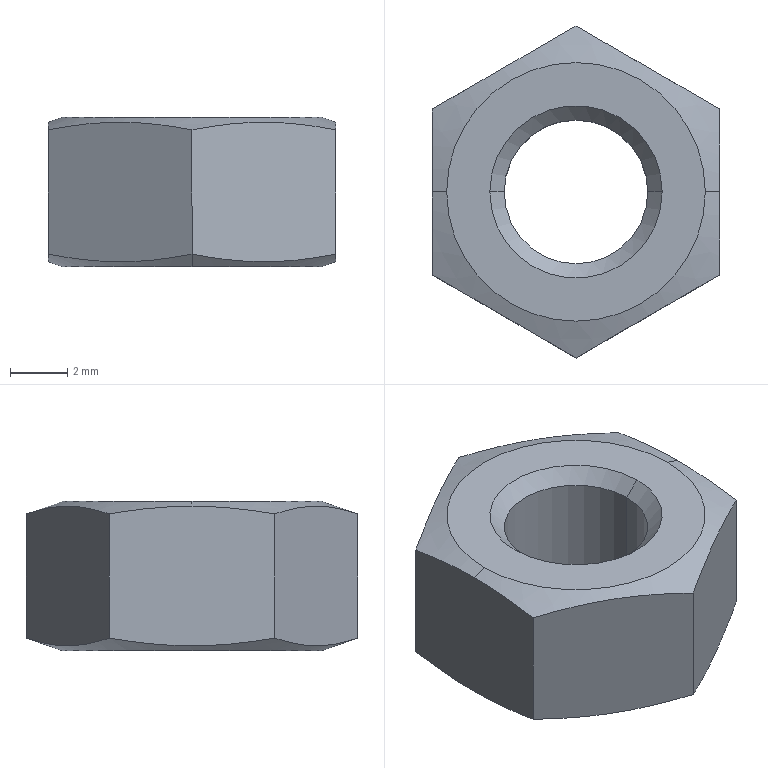Part | STEP file | 921271102 | 1 solid | 18 faces | box 10 x 11.547 x 5.2 mm | volume 337.323 mm3 | cone 8 | plane 8 | cylinder 2 | commonest cylinder face diameters 5 x2
STEP:
#1=CARTESIAN_POINT('',(2.5,0.,4.7));
#2=VERTEX_POINT('',#1);
#3=CARTESIAN_POINT('',(-2.5,0.,4.7));
#4=VERTEX_POINT('',#3);
#5=CARTESIAN_POINT('',(0.,0.,4.7));
#6=DIRECTION('',(0.,0.,-1.));
#7=DIRECTION('',(-1.,0.,0.));
#8=AXIS2_PLACEMENT_3D('',#5,#6,#7);
#9=CIRCLE('',#8,2.5);
#10=EDGE_CURVE('',#2,#4,#9,.T.);
#11=ORIENTED_EDGE('',*,*,#10,.F.);
#12=CARTESIAN_POINT('',(2.5,0.,0.5));
#13=VERTEX_POINT('',#12);
#14=CARTESIAN_POINT('',(2.5,0.,5.2));
#15=DIRECTION('',(0.,0.,-1.));
#16=VECTOR('',#15,1000.);
#17=LINE('',#14,#16);
#18=EDGE_CURVE('',#2,#13,#17,.T.);
#19=ORIENTED_EDGE('',*,*,#18,.T.);
#20=CARTESIAN_POINT('',(-2.5,0.,0.5));
#21=VERTEX_POINT('',#20);
#22=CARTESIAN_POINT('',(0.,0.,0.5));
#23=DIRECTION('',(0.,0.,1.));
#24=DIRECTION('',(-1.,0.,0.));
#25=AXIS2_PLACEMENT_3D('',#22,#23,#24);
#26=CIRCLE('',#25,2.5);
#27=EDGE_CURVE('',#21,#13,#26,.T.);
#28=ORIENTED_EDGE('',*,*,#27,.F.);
#29=CARTESIAN_POINT('',(-2.5,0.,5.2));
#30=DIRECTION('',(0.,0.,-1.));
#31=VECTOR('',#30,1000.);
#32=LINE('',#29,#31);
#33=EDGE_CURVE('',#4,#21,#32,.T.);
#34=ORIENTED_EDGE('',*,*,#33,.F.);
#35=EDGE_LOOP('',(#11,#19,#28,#34));
#36=FACE_OUTER_BOUND('',#35,.T.);
#37=CARTESIAN_POINT('',(0.,0.,5.2));
#38=DIRECTION('',(0.,0.,-1.));
#39=DIRECTION('',(-1.,0.,0.));
#40=AXIS2_PLACEMENT_3D('',#37,#38,#39);
#41=CYLINDRICAL_SURFACE('',#40,2.5);
#42=ADVANCED_FACE('',(#36),#41,.F.);
#43=ORIENTED_EDGE('',*,*,#10,.T.);
#44=CARTESIAN_POINT('',(-3.,0.,5.2));
#45=VERTEX_POINT('',#44);
#46=CARTESIAN_POINT('',(-3.,0.,5.2));
#47=DIRECTION('',(-0.7071,0.,0.7071));
#48=VECTOR('',#47,1000.);
#49=LINE('',#46,#48);
#50=EDGE_CURVE('',#4,#45,#49,.T.);
#51=ORIENTED_EDGE('',*,*,#50,.T.);
#52=CARTESIAN_POINT('',(3.,0.,5.2));
#53=VERTEX_POINT('',#52);
#54=CARTESIAN_POINT('',(0.,0.,5.2));
#55=DIRECTION('',(0.,0.,-1.));
#56=DIRECTION('',(1.,0.,0.));
#57=AXIS2_PLACEMENT_3D('',#54,#55,#56);
#58=CIRCLE('',#57,3.);
#59=EDGE_CURVE('',#53,#45,#58,.T.);
#60=ORIENTED_EDGE('',*,*,#59,.F.);
#61=CARTESIAN_POINT('',(3.,0.,5.2));
#62=DIRECTION('',(0.7071,0.,0.7071));
#63=VECTOR('',#62,1000.);
#64=LINE('',#61,#63);
#65=EDGE_CURVE('',#2,#53,#64,.T.);
#66=ORIENTED_EDGE('',*,*,#65,.F.);
#67=EDGE_LOOP('',(#43,#51,#60,#66));
#68=FACE_OUTER_BOUND('',#67,.T.);
#69=CARTESIAN_POINT('',(0.,0.,5.2));
#70=DIRECTION('',(0.,0.,1.));
#71=DIRECTION('',(1.,0.,0.));
#72=AXIS2_PLACEMENT_3D('',#69,#70,#71);
#73=CONICAL_SURFACE('',#72,3.,0.7854);
#74=ADVANCED_FACE('',(#68),#73,.F.);
#75=ORIENTED_EDGE('',*,*,#27,.T.);
#76=CARTESIAN_POINT('',(3.,0.,0.));
#77=VERTEX_POINT('',#76);
#78=CARTESIAN_POINT('',(3.,0.,0.));
#79=DIRECTION('',(0.7071,0.,-0.7071));
#80=VECTOR('',#79,1000.);
#81=LINE('',#78,#80);
#82=EDGE_CURVE('',#13,#77,#81,.T.);
#83=ORIENTED_EDGE('',*,*,#82,.T.);
#84=CARTESIAN_POINT('',(-3.,0.,0.));
#85=VERTEX_POINT('',#84);
#86=CARTESIAN_POINT('',(0.,0.,0.));
#87=DIRECTION('',(0.,0.,1.));
#88=DIRECTION('',(-1.,0.,0.));
#89=AXIS2_PLACEMENT_3D('',#86,#87,#88);
#90=CIRCLE('',#89,3.);
#91=EDGE_CURVE('',#85,#77,#90,.T.);
#92=ORIENTED_EDGE('',*,*,#91,.F.);
#93=CARTESIAN_POINT('',(-3.,0.,0.));
#94=DIRECTION('',(-0.7071,0.,-0.7071));
#95=VECTOR('',#94,1000.);
#96=LINE('',#93,#95);
#97=EDGE_CURVE('',#21,#85,#96,.T.);
#98=ORIENTED_EDGE('',*,*,#97,.F.);
#99=EDGE_LOOP('',(#75,#83,#92,#98));
#100=FACE_OUTER_BOUND('',#99,.T.);
#101=CARTESIAN_POINT('',(0.,0.,0.));
#102=DIRECTION('',(0.,0.,-1.));
#103=DIRECTION('',(-1.,0.,0.));
#104=AXIS2_PLACEMENT_3D('',#101,#102,#103);
#105=CONICAL_SURFACE('',#104,3.,0.7854);
#106=ADVANCED_FACE('',(#100),#105,.F.);
#107=CARTESIAN_POINT('',(4.5,0.,5.2));
#108=VERTEX_POINT('',#107);
#109=CARTESIAN_POINT('',(-4.5,0.,5.2));
#110=VERTEX_POINT('',#109);
#111=CARTESIAN_POINT('',(0.,0.,5.2));
#112=DIRECTION('',(0.,0.,1.));
#113=DIRECTION('',(-1.,0.,0.));
#114=AXIS2_PLACEMENT_3D('',#111,#112,#113);
#115=CIRCLE('',#114,4.5);
#116=EDGE_CURVE('',#108,#110,#115,.T.);
#117=ORIENTED_EDGE('',*,*,#116,.F.);
#118=CARTESIAN_POINT('',(5.,0.,5.028));
#119=VERTEX_POINT('',#118);
#120=CARTESIAN_POINT('',(5.781,0.,4.759));
#121=DIRECTION('',(0.9455,0.,-0.3256));
#122=VECTOR('',#121,1000.);
#123=LINE('',#120,#122);
#124=EDGE_CURVE('',#108,#119,#123,.T.);
#125=ORIENTED_EDGE('',*,*,#124,.T.);
#126=CARTESIAN_POINT('',(5.,2.887,4.761));
#127=VERTEX_POINT('',#126);
#128=CARTESIAN_POINT('',(5.,0.,5.028));
#129=CARTESIAN_POINT('',(5.,0.9623,5.028));
#130=CARTESIAN_POINT('',(5.,1.925,4.927));
#131=CARTESIAN_POINT('',(5.,2.887,4.761));
#132=B_SPLINE_CURVE_WITH_KNOTS('',3,(#128,#129,#130,#131),.UNSPECIFIED.,.F.,.F.,(4,4),(0.002887,0.005774),.UNSPECIFIED.);
#133=EDGE_CURVE('',#119,#127,#132,.T.);
#134=ORIENTED_EDGE('',*,*,#133,.T.);
#135=CARTESIAN_POINT('',(0.000000041,5.774,4.761));
#136=VERTEX_POINT('',#135);
#137=CARTESIAN_POINT('',(5.,2.887,4.761));
#138=CARTESIAN_POINT('',(4.167,3.368,4.927));
#139=CARTESIAN_POINT('',(2.5,4.33,5.129));
#140=CARTESIAN_POINT('',(0.8333,5.292,4.927));
#141=CARTESIAN_POINT('',(0.000000041,5.774,4.761));
#142=B_SPLINE_CURVE_WITH_KNOTS('',3,(#137,#138,#139,#140,#141),.UNSPECIFIED.,.F.,.F.,(4,1,4),(0.,0.002887,0.005774),.UNSPECIFIED.);
#143=EDGE_CURVE('',#127,#136,#142,.T.);
#144=ORIENTED_EDGE('',*,*,#143,.T.);
#145=CARTESIAN_POINT('',(-5.,2.887,4.761));
#146=VERTEX_POINT('',#145);
#147=CARTESIAN_POINT('',(0.000000041,5.774,4.761));
#148=CARTESIAN_POINT('',(-0.8333,5.292,4.927));
#149=CARTESIAN_POINT('',(-2.5,4.33,5.129));
#150=CARTESIAN_POINT('',(-4.167,3.368,4.927));
#151=CARTESIAN_POINT('',(-5.,2.887,4.761));
#152=B_SPLINE_CURVE_WITH_KNOTS('',3,(#147,#148,#149,#150,#151),.UNSPECIFIED.,.F.,.F.,(4,1,4),(0.,0.002887,0.005774),.UNSPECIFIED.);
#153=EDGE_CURVE('',#136,#146,#152,.T.);
#154=ORIENTED_EDGE('',*,*,#153,.T.);
#155=CARTESIAN_POINT('',(-5.,0.,5.028));
#156=VERTEX_POINT('',#155);
#157=CARTESIAN_POINT('',(-5.,2.887,4.761));
#158=CARTESIAN_POINT('',(-5.,1.925,4.927));
#159=CARTESIAN_POINT('',(-5.,0.9623,5.028));
#160=CARTESIAN_POINT('',(-5.,0.,5.028));
#161=B_SPLINE_CURVE_WITH_KNOTS('',3,(#157,#158,#159,#160),.UNSPECIFIED.,.F.,.F.,(4,4),(0.,0.002887),.UNSPECIFIED.);
#162=EDGE_CURVE('',#146,#156,#161,.T.);
#163=ORIENTED_EDGE('',*,*,#162,.T.);
#164=CARTESIAN_POINT('',(-5.781,0.,4.759));
#165=DIRECTION('',(-0.9455,0.,-0.3256));
#166=VECTOR('',#165,1000.);
#167=LINE('',#164,#166);
#168=EDGE_CURVE('',#110,#156,#167,.T.);
#169=ORIENTED_EDGE('',*,*,#168,.F.);
#170=EDGE_LOOP('',(#117,#125,#134,#144,#154,#163,#169));
#171=FACE_OUTER_BOUND('',#170,.T.);
#172=CARTESIAN_POINT('',(0.,0.,4.759));
#173=DIRECTION('',(0.,0.,-1.));
#174=DIRECTION('',(-1.,0.,0.));
#175=AXIS2_PLACEMENT_3D('',#172,#173,#174);
#176=CONICAL_SURFACE('',#175,5.781,1.239);
#177=ADVANCED_FACE('',(#171),#176,.T.);
#178=CARTESIAN_POINT('',(0.,-4.5,0.));
#179=VERTEX_POINT('',#178);
#180=CARTESIAN_POINT('',(0.,4.5,0.));
#181=VERTEX_POINT('',#180);
#182=CARTESIAN_POINT('',(0.,0.,0.));
#183=DIRECTION('',(0.,0.,1.));
#184=DIRECTION('',(0.,-1.,0.));
#185=AXIS2_PLACEMENT_3D('',#182,#183,#184);
#186=CIRCLE('',#185,4.5);
#187=EDGE_CURVE('',#179,#181,#186,.T.);
#188=ORIENTED_EDGE('',*,*,#187,.T.);
#189=CARTESIAN_POINT('',(-0.000000041,5.774,0.4385));
#190=VERTEX_POINT('',#189);
#191=CARTESIAN_POINT('',(0.,5.781,0.4411));
#192=DIRECTION('',(0.,0.9455,0.3256));
#193=VECTOR('',#192,1000.);
#194=LINE('',#191,#193);
#195=EDGE_CURVE('',#181,#190,#194,.T.);
#196=ORIENTED_EDGE('',*,*,#195,.T.);
#197=CARTESIAN_POINT('',(5.,2.887,0.4385));
#198=VERTEX_POINT('',#197);
#199=CARTESIAN_POINT('',(-0.000000041,5.774,0.4385));
#200=CARTESIAN_POINT('',(0.8333,5.292,0.2728));
#201=CARTESIAN_POINT('',(2.5,4.33,0.07149));
#202=CARTESIAN_POINT('',(4.167,3.368,0.2728));
#203=CARTESIAN_POINT('',(5.,2.887,0.4385));
#204=B_SPLINE_CURVE_WITH_KNOTS('',3,(#199,#200,#201,#202,#203),.UNSPECIFIED.,.F.,.F.,(4,1,4),(0.,0.002887,0.005774),.UNSPECIFIED.);
#205=EDGE_CURVE('',#190,#198,#204,.T.);
#206=ORIENTED_EDGE('',*,*,#205,.T.);
#207=CARTESIAN_POINT('',(5.,-2.887,0.4385));
#208=VERTEX_POINT('',#207);
#209=CARTESIAN_POINT('',(5.,2.887,0.4385));
#210=CARTESIAN_POINT('',(5.,1.925,0.2728));
#211=CARTESIAN_POINT('',(5.,0.000000063,0.07149));
#212=CARTESIAN_POINT('',(5.,-1.925,0.2728));
#213=CARTESIAN_POINT('',(5.,-2.887,0.4385));
#214=B_SPLINE_CURVE_WITH_KNOTS('',3,(#209,#210,#211,#212,#213),.UNSPECIFIED.,.F.,.F.,(4,1,4),(0.,0.002887,0.005774),.UNSPECIFIED.);
#215=EDGE_CURVE('',#198,#208,#214,.T.);
#216=ORIENTED_EDGE('',*,*,#215,.T.);
#217=CARTESIAN_POINT('',(0.000000011,-5.774,0.4385));
#218=VERTEX_POINT('',#217);
#219=CARTESIAN_POINT('',(5.,-2.887,0.4385));
#220=CARTESIAN_POINT('',(4.167,-3.368,0.2728));
#221=CARTESIAN_POINT('',(2.5,-4.33,0.07149));
#222=CARTESIAN_POINT('',(0.8333,-5.292,0.2728));
#223=CARTESIAN_POINT('',(0.000000011,-5.774,0.4385));
#224=B_SPLINE_CURVE_WITH_KNOTS('',3,(#219,#220,#221,#222,#223),.UNSPECIFIED.,.F.,.F.,(4,1,4),(0.,0.002887,0.005774),.UNSPECIFIED.);
#225=EDGE_CURVE('',#208,#218,#224,.T.);
#226=ORIENTED_EDGE('',*,*,#225,.T.);
#227=CARTESIAN_POINT('',(0.,-5.781,0.4411));
#228=DIRECTION('',(0.,-0.9455,0.3256));
#229=VECTOR('',#228,1000.);
#230=LINE('',#227,#229);
#231=EDGE_CURVE('',#179,#218,#230,.T.);
#232=ORIENTED_EDGE('',*,*,#231,.F.);
#233=EDGE_LOOP('',(#188,#196,#206,#216,#226,#232));
#234=FACE_OUTER_BOUND('',#233,.T.);
#235=CARTESIAN_POINT('',(0.,0.,0.4411));
#236=DIRECTION('',(0.,0.,1.));
#237=DIRECTION('',(0.,-1.,0.));
#238=AXIS2_PLACEMENT_3D('',#235,#236,#237);
#239=CONICAL_SURFACE('',#238,5.781,1.239);
#240=ADVANCED_FACE('',(#234),#239,.T.);
#241=ORIENTED_EDGE('',*,*,#18,.F.);
#242=CARTESIAN_POINT('',(0.,0.,4.7));
#243=DIRECTION('',(0.,0.,-1.));
#244=DIRECTION('',(-1.,0.,0.));
#245=AXIS2_PLACEMENT_3D('',#242,#243,#244);
#246=CIRCLE('',#245,2.5);
#247=EDGE_CURVE('',#4,#2,#246,.T.);
#248=ORIENTED_EDGE('',*,*,#247,.F.);
#249=ORIENTED_EDGE('',*,*,#33,.T.);
#250=CARTESIAN_POINT('',(0.,0.,0.5));
#251=DIRECTION('',(0.,0.,1.));
#252=DIRECTION('',(-1.,0.,0.));
#253=AXIS2_PLACEMENT_3D('',#250,#251,#252);
#254=CIRCLE('',#253,2.5);
#255=EDGE_CURVE('',#13,#21,#254,.T.);
#256=ORIENTED_EDGE('',*,*,#255,.F.);
#257=EDGE_LOOP('',(#241,#248,#249,#256));
#258=FACE_OUTER_BOUND('',#257,.T.);
#259=CARTESIAN_POINT('',(0.,0.,5.2));
#260=DIRECTION('',(0.,0.,-1.));
#261=DIRECTION('',(-1.,0.,0.));
#262=AXIS2_PLACEMENT_3D('',#259,#260,#261);
#263=CYLINDRICAL_SURFACE('',#262,2.5);
#264=ADVANCED_FACE('',(#258),#263,.F.);
#265=ORIENTED_EDGE('',*,*,#50,.F.);
#266=ORIENTED_EDGE('',*,*,#247,.T.);
#267=ORIENTED_EDGE('',*,*,#65,.T.);
#268=CARTESIAN_POINT('',(0.,0.,5.2));
#269=DIRECTION('',(0.,0.,-1.));
#270=DIRECTION('',(1.,0.,0.));
#271=AXIS2_PLACEMENT_3D('',#268,#269,#270);
#272=CIRCLE('',#271,3.);
#273=EDGE_CURVE('',#45,#53,#272,.T.);
#274=ORIENTED_EDGE('',*,*,#273,.F.);
#275=EDGE_LOOP('',(#265,#266,#267,#274));
#276=FACE_OUTER_BOUND('',#275,.T.);
#277=CARTESIAN_POINT('',(0.,0.,5.2));
#278=DIRECTION('',(0.,0.,1.));
#279=DIRECTION('',(1.,0.,0.));
#280=AXIS2_PLACEMENT_3D('',#277,#278,#279);
#281=CONICAL_SURFACE('',#280,3.,0.7854);
#282=ADVANCED_FACE('',(#276),#281,.F.);
#283=ORIENTED_EDGE('',*,*,#82,.F.);
#284=ORIENTED_EDGE('',*,*,#255,.T.);
#285=ORIENTED_EDGE('',*,*,#97,.T.);
#286=CARTESIAN_POINT('',(0.,0.,0.));
#287=DIRECTION('',(0.,0.,1.));
#288=DIRECTION('',(-1.,0.,0.));
#289=AXIS2_PLACEMENT_3D('',#286,#287,#288);
#290=CIRCLE('',#289,3.);
#291=EDGE_CURVE('',#77,#85,#290,.T.);
#292=ORIENTED_EDGE('',*,*,#291,.F.);
#293=EDGE_LOOP('',(#283,#284,#285,#292));
#294=FACE_OUTER_BOUND('',#293,.T.);
#295=CARTESIAN_POINT('',(0.,0.,0.));
#296=DIRECTION('',(0.,0.,-1.));
#297=DIRECTION('',(-1.,0.,0.));
#298=AXIS2_PLACEMENT_3D('',#295,#296,#297);
#299=CONICAL_SURFACE('',#298,3.,0.7854);
#300=ADVANCED_FACE('',(#294),#299,.F.);
#301=ORIENTED_EDGE('',*,*,#59,.T.);
#302=ORIENTED_EDGE('',*,*,#273,.T.);
#303=EDGE_LOOP('',(#301,#302));
#304=FACE_BOUND('',#303,.T.);
#305=CARTESIAN_POINT('',(0.,0.,5.2));
#306=DIRECTION('',(0.,0.,1.));
#307=DIRECTION('',(-1.,0.,0.));
#308=AXIS2_PLACEMENT_3D('',#305,#306,#307);
#309=CIRCLE('',#308,4.5);
#310=EDGE_CURVE('',#110,#108,#309,.T.);
#311=ORIENTED_EDGE('',*,*,#310,.T.);
#312=ORIENTED_EDGE('',*,*,#116,.T.);
#313=EDGE_LOOP('',(#311,#312));
#314=FACE_OUTER_BOUND('',#313,.T.);
#315=CARTESIAN_POINT('',(-5.,-2.887,5.2));
#316=DIRECTION('',(0.,0.,1.));
#317=DIRECTION('',(1.,0.,0.));
#318=AXIS2_PLACEMENT_3D('',#315,#316,#317);
#319=PLANE('',#318);
#320=ADVANCED_FACE('',(#304,#314),#319,.T.);
#321=ORIENTED_EDGE('',*,*,#187,.F.);
#322=CARTESIAN_POINT('',(0.,0.,0.));
#323=DIRECTION('',(0.,0.,1.));
#324=DIRECTION('',(0.,-1.,0.));
#325=AXIS2_PLACEMENT_3D('',#322,#323,#324);
#326=CIRCLE('',#325,4.5);
#327=EDGE_CURVE('',#181,#179,#326,.T.);
#328=ORIENTED_EDGE('',*,*,#327,.F.);
#329=EDGE_LOOP('',(#321,#328));
#330=FACE_OUTER_BOUND('',#329,.T.);
#331=ORIENTED_EDGE('',*,*,#91,.T.);
#332=ORIENTED_EDGE('',*,*,#291,.T.);
#333=EDGE_LOOP('',(#331,#332));
#334=FACE_BOUND('',#333,.T.);
#335=CARTESIAN_POINT('',(-5.,-2.887,0.));
#336=DIRECTION('',(0.,0.,1.));
#337=DIRECTION('',(1.,0.,0.));
#338=AXIS2_PLACEMENT_3D('',#335,#336,#337);
#339=PLANE('',#338);
#340=ADVANCED_FACE('',(#330,#334),#339,.F.);
#341=ORIENTED_EDGE('',*,*,#124,.F.);
#342=ORIENTED_EDGE('',*,*,#310,.F.);
#343=ORIENTED_EDGE('',*,*,#168,.T.);
#344=CARTESIAN_POINT('',(-5.,-2.887,4.761));
#345=VERTEX_POINT('',#344);
#346=CARTESIAN_POINT('',(-5.,0.,5.028));
#347=CARTESIAN_POINT('',(-5.,-0.9623,5.028));
#348=CARTESIAN_POINT('',(-5.,-1.925,4.927));
#349=CARTESIAN_POINT('',(-5.,-2.887,4.761));
#350=B_SPLINE_CURVE_WITH_KNOTS('',3,(#346,#347,#348,#349),.UNSPECIFIED.,.F.,.F.,(4,4),(0.002887,0.005774),.UNSPECIFIED.);
#351=EDGE_CURVE('',#156,#345,#350,.T.);
#352=ORIENTED_EDGE('',*,*,#351,.T.);
#353=CARTESIAN_POINT('',(-0.000000041,-5.774,4.761));
#354=VERTEX_POINT('',#353);
#355=CARTESIAN_POINT('',(-5.,-2.887,4.761));
#356=CARTESIAN_POINT('',(-4.167,-3.368,4.927));
#357=CARTESIAN_POINT('',(-2.5,-4.33,5.129));
#358=CARTESIAN_POINT('',(-0.8333,-5.292,4.927));
#359=CARTESIAN_POINT('',(-0.000000041,-5.774,4.761));
#360=B_SPLINE_CURVE_WITH_KNOTS('',3,(#355,#356,#357,#358,#359),.UNSPECIFIED.,.F.,.F.,(4,1,4),(0.,0.002887,0.005774),.UNSPECIFIED.);
#361=EDGE_CURVE('',#345,#354,#360,.T.);
#362=ORIENTED_EDGE('',*,*,#361,.T.);
#363=CARTESIAN_POINT('',(5.,-2.887,4.761));
#364=VERTEX_POINT('',#363);
#365=CARTESIAN_POINT('',(-0.000000041,-5.774,4.761));
#366=CARTESIAN_POINT('',(0.8333,-5.292,4.927));
#367=CARTESIAN_POINT('',(2.5,-4.33,5.129));
#368=CARTESIAN_POINT('',(4.167,-3.368,4.927));
#369=CARTESIAN_POINT('',(5.,-2.887,4.761));
#370=B_SPLINE_CURVE_WITH_KNOTS('',3,(#365,#366,#367,#368,#369),.UNSPECIFIED.,.F.,.F.,(4,1,4),(0.,0.002887,0.005774),.UNSPECIFIED.);
#371=EDGE_CURVE('',#354,#364,#370,.T.);
#372=ORIENTED_EDGE('',*,*,#371,.T.);
#373=CARTESIAN_POINT('',(5.,-2.887,4.761));
#374=CARTESIAN_POINT('',(5.,-1.925,4.927));
#375=CARTESIAN_POINT('',(5.,-0.9623,5.028));
#376=CARTESIAN_POINT('',(5.,0.,5.028));
#377=B_SPLINE_CURVE_WITH_KNOTS('',3,(#373,#374,#375,#376),.UNSPECIFIED.,.F.,.F.,(4,4),(0.,0.002887),.UNSPECIFIED.);
#378=EDGE_CURVE('',#364,#119,#377,.T.);
#379=ORIENTED_EDGE('',*,*,#378,.T.);
#380=EDGE_LOOP('',(#341,#342,#343,#352,#362,#372,#379));
#381=FACE_OUTER_BOUND('',#380,.T.);
#382=CARTESIAN_POINT('',(0.,0.,4.759));
#383=DIRECTION('',(0.,0.,-1.));
#384=DIRECTION('',(-1.,0.,0.));
#385=AXIS2_PLACEMENT_3D('',#382,#383,#384);
#386=CONICAL_SURFACE('',#385,5.781,1.239);
#387=ADVANCED_FACE('',(#381),#386,.T.);
#388=ORIENTED_EDGE('',*,*,#195,.F.);
#389=ORIENTED_EDGE('',*,*,#327,.T.);
#390=ORIENTED_EDGE('',*,*,#231,.T.);
#391=CARTESIAN_POINT('',(-5.,-2.887,0.4385));
#392=VERTEX_POINT('',#391);
#393=CARTESIAN_POINT('',(0.000000011,-5.774,0.4385));
#394=CARTESIAN_POINT('',(-0.8333,-5.292,0.2728));
#395=CARTESIAN_POINT('',(-2.5,-4.33,0.07149));
#396=CARTESIAN_POINT('',(-4.167,-3.368,0.2728));
#397=CARTESIAN_POINT('',(-5.,-2.887,0.4385));
#398=B_SPLINE_CURVE_WITH_KNOTS('',3,(#393,#394,#395,#396,#397),.UNSPECIFIED.,.F.,.F.,(4,1,4),(0.,0.002887,0.005774),.UNSPECIFIED.);
#399=EDGE_CURVE('',#218,#392,#398,.T.);
#400=ORIENTED_EDGE('',*,*,#399,.T.);
#401=CARTESIAN_POINT('',(-5.,2.887,0.4385));
#402=VERTEX_POINT('',#401);
#403=CARTESIAN_POINT('',(-5.,-2.887,0.4385));
#404=CARTESIAN_POINT('',(-5.,-1.925,0.2728));
#405=CARTESIAN_POINT('',(-5.,0.,0.07149));
#406=CARTESIAN_POINT('',(-5.,1.925,0.2728));
#407=CARTESIAN_POINT('',(-5.,2.887,0.4385));
#408=B_SPLINE_CURVE_WITH_KNOTS('',3,(#403,#404,#405,#406,#407),.UNSPECIFIED.,.F.,.F.,(4,1,4),(0.,0.002887,0.005774),.UNSPECIFIED.);
#409=EDGE_CURVE('',#392,#402,#408,.T.);
#410=ORIENTED_EDGE('',*,*,#409,.T.);
#411=CARTESIAN_POINT('',(-5.,2.887,0.4385));
#412=CARTESIAN_POINT('',(-4.167,3.368,0.2728));
#413=CARTESIAN_POINT('',(-2.5,4.33,0.07149));
#414=CARTESIAN_POINT('',(-0.8333,5.292,0.2728));
#415=CARTESIAN_POINT('',(-0.000000041,5.774,0.4385));
#416=B_SPLINE_CURVE_WITH_KNOTS('',3,(#411,#412,#413,#414,#415),.UNSPECIFIED.,.F.,.F.,(4,1,4),(0.,0.002887,0.005774),.UNSPECIFIED.);
#417=EDGE_CURVE('',#402,#190,#416,.T.);
#418=ORIENTED_EDGE('',*,*,#417,.T.);
#419=EDGE_LOOP('',(#388,#389,#390,#400,#410,#418));
#420=FACE_OUTER_BOUND('',#419,.T.);
#421=CARTESIAN_POINT('',(0.,0.,0.4411));
#422=DIRECTION('',(0.,0.,1.));
#423=DIRECTION('',(0.,-1.,0.));
#424=AXIS2_PLACEMENT_3D('',#421,#422,#423);
#425=CONICAL_SURFACE('',#424,5.781,1.239);
#426=ADVANCED_FACE('',(#420),#425,.T.);
#427=ORIENTED_EDGE('',*,*,#162,.F.);
#428=CARTESIAN_POINT('',(-5.,2.887,5.2));
#429=DIRECTION('',(0.,0.,1.));
#430=VECTOR('',#429,1000.);
#431=LINE('',#428,#430);
#432=EDGE_CURVE('',#402,#146,#431,.T.);
#433=ORIENTED_EDGE('',*,*,#432,.F.);
#434=ORIENTED_EDGE('',*,*,#409,.F.);
#435=CARTESIAN_POINT('',(-5.,-2.887,5.2));
#436=DIRECTION('',(0.,0.,-1.));
#437=VECTOR('',#436,1000.);
#438=LINE('',#435,#437);
#439=EDGE_CURVE('',#345,#392,#438,.T.);
#440=ORIENTED_EDGE('',*,*,#439,.F.);
#441=ORIENTED_EDGE('',*,*,#351,.F.);
#442=EDGE_LOOP('',(#427,#433,#434,#440,#441));
#443=FACE_OUTER_BOUND('',#442,.T.);
#444=CARTESIAN_POINT('',(-5.,2.887,5.2));
#445=DIRECTION('',(1.,0.,0.));
#446=DIRECTION('',(0.,1.,0.));
#447=AXIS2_PLACEMENT_3D('',#444,#445,#446);
#448=PLANE('',#447);
#449=ADVANCED_FACE('',(#443),#448,.F.);
#450=ORIENTED_EDGE('',*,*,#153,.F.);
#451=CARTESIAN_POINT('',(0.,5.774,5.2));
#452=DIRECTION('',(0.,0.,1.));
#453=VECTOR('',#452,1000.);
#454=LINE('',#451,#453);
#455=EDGE_CURVE('',#190,#136,#454,.T.);
#456=ORIENTED_EDGE('',*,*,#455,.F.);
#457=ORIENTED_EDGE('',*,*,#417,.F.);
#458=ORIENTED_EDGE('',*,*,#432,.T.);
#459=EDGE_LOOP('',(#450,#456,#457,#458));
#460=FACE_OUTER_BOUND('',#459,.T.);
#461=CARTESIAN_POINT('',(0.,5.774,5.2));
#462=DIRECTION('',(0.5,-0.866,0.));
#463=DIRECTION('',(0.866,0.5,0.));
#464=AXIS2_PLACEMENT_3D('',#461,#462,#463);
#465=PLANE('',#464);
#466=ADVANCED_FACE('',(#460),#465,.F.);
#467=ORIENTED_EDGE('',*,*,#143,.F.);
#468=CARTESIAN_POINT('',(5.,2.887,5.2));
#469=DIRECTION('',(0.,0.,1.));
#470=VECTOR('',#469,1000.);
#471=LINE('',#468,#470);
#472=EDGE_CURVE('',#198,#127,#471,.T.);
#473=ORIENTED_EDGE('',*,*,#472,.F.);
#474=ORIENTED_EDGE('',*,*,#205,.F.);
#475=ORIENTED_EDGE('',*,*,#455,.T.);
#476=EDGE_LOOP('',(#467,#473,#474,#475));
#477=FACE_OUTER_BOUND('',#476,.T.);
#478=CARTESIAN_POINT('',(5.,2.887,5.2));
#479=DIRECTION('',(-0.5,-0.866,0.));
#480=DIRECTION('',(0.866,-0.5,0.));
#481=AXIS2_PLACEMENT_3D('',#478,#479,#480);
#482=PLANE('',#481);
#483=ADVANCED_FACE('',(#477),#482,.F.);
#484=ORIENTED_EDGE('',*,*,#378,.F.);
#485=CARTESIAN_POINT('',(5.,-2.887,5.2));
#486=DIRECTION('',(0.,0.,1.));
#487=VECTOR('',#486,1000.);
#488=LINE('',#485,#487);
#489=EDGE_CURVE('',#208,#364,#488,.T.);
#490=ORIENTED_EDGE('',*,*,#489,.F.);
#491=ORIENTED_EDGE('',*,*,#215,.F.);
#492=ORIENTED_EDGE('',*,*,#472,.T.);
#493=ORIENTED_EDGE('',*,*,#133,.F.);
#494=EDGE_LOOP('',(#484,#490,#491,#492,#493));
#495=FACE_OUTER_BOUND('',#494,.T.);
#496=CARTESIAN_POINT('',(5.,-2.887,5.2));
#497=DIRECTION('',(-1.,0.,0.));
#498=DIRECTION('',(0.,-1.,0.));
#499=AXIS2_PLACEMENT_3D('',#496,#497,#498);
#500=PLANE('',#499);
#501=ADVANCED_FACE('',(#495),#500,.F.);
#502=ORIENTED_EDGE('',*,*,#371,.F.);
#503=CARTESIAN_POINT('',(0.,-5.774,5.2));
#504=DIRECTION('',(0.,0.,1.));
#505=VECTOR('',#504,1000.);
#506=LINE('',#503,#505);
#507=EDGE_CURVE('',#218,#354,#506,.T.);
#508=ORIENTED_EDGE('',*,*,#507,.F.);
#509=ORIENTED_EDGE('',*,*,#225,.F.);
#510=ORIENTED_EDGE('',*,*,#489,.T.);
#511=EDGE_LOOP('',(#502,#508,#509,#510));
#512=FACE_OUTER_BOUND('',#511,.T.);
#513=CARTESIAN_POINT('',(0.,-5.774,5.2));
#514=DIRECTION('',(-0.5,0.866,0.));
#515=DIRECTION('',(-0.866,-0.5,0.));
#516=AXIS2_PLACEMENT_3D('',#513,#514,#515);
#517=PLANE('',#516);
#518=ADVANCED_FACE('',(#512),#517,.F.);
#519=ORIENTED_EDGE('',*,*,#361,.F.);
#520=ORIENTED_EDGE('',*,*,#439,.T.);
#521=ORIENTED_EDGE('',*,*,#399,.F.);
#522=ORIENTED_EDGE('',*,*,#507,.T.);
#523=EDGE_LOOP('',(#519,#520,#521,#522));
#524=FACE_OUTER_BOUND('',#523,.T.);
#525=CARTESIAN_POINT('',(-5.,-2.887,5.2));
#526=DIRECTION('',(0.5,0.866,0.));
#527=DIRECTION('',(-0.866,0.5,0.));
#528=AXIS2_PLACEMENT_3D('',#525,#526,#527);
#529=PLANE('',#528);
#530=ADVANCED_FACE('',(#524),#529,.F.);
#531=CLOSED_SHELL('',(#42,#74,#106,#177,#240,#264,#282,#300,#320,#340,#387,#426,#449,#466,#483,#501,#518,#530));
#532=MANIFOLD_SOLID_BREP('',#531);
#533=CARTESIAN_POINT('',(0.,0.,0.));
#534=DIRECTION('',(0.,0.,1.));
#535=DIRECTION('',(1.,0.,0.));
#536=AXIS2_PLACEMENT_3D('',#533,#534,#535);
#537=(LENGTH_UNIT()NAMED_UNIT(*)SI_UNIT(.MILLI.,.METRE.));
#538=UNCERTAINTY_MEASURE_WITH_UNIT(LENGTH_MEASURE(0.00001),#537,'','');
#539=(NAMED_UNIT(*)PLANE_ANGLE_UNIT()SI_UNIT($,.RADIAN.));
#540=(NAMED_UNIT(*)SI_UNIT($,.STERADIAN.)SOLID_ANGLE_UNIT());
#541=(GEOMETRIC_REPRESENTATION_CONTEXT(3)GLOBAL_UNCERTAINTY_ASSIGNED_CONTEXT((#538))GLOBAL_UNIT_ASSIGNED_CONTEXT((#537,#539,#540))REPRESENTATION_CONTEXT('',''));
#542=ADVANCED_BREP_SHAPE_REPRESENTATION('',(#532,#536),#541);